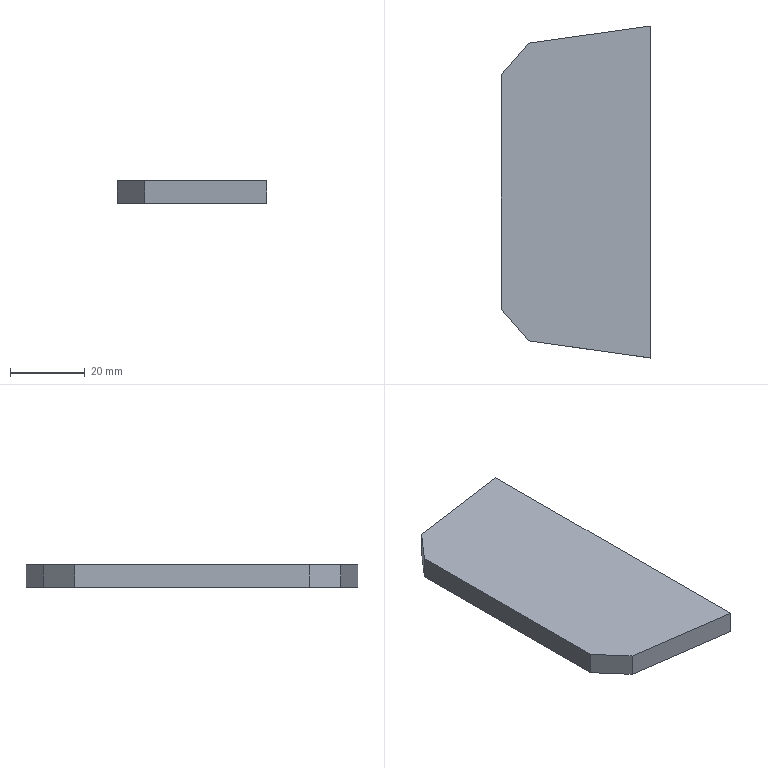Part | SolidWorks | features Extrusion 1 | 1 solid | 8 faces | box 40 x 88.903 x 6 mm | volume 19663 mm3 | plane 8
STEP:
#1=CARTESIAN_POINT('',(-4.,-5.549,0.));
#2=VERTEX_POINT('',#1);
#3=CARTESIAN_POINT('',(-4.,-94.451,0.));
#4=VERTEX_POINT('',#3);
#5=CARTESIAN_POINT('',(-4.,-5.549,0.));
#6=DIRECTION('',(0.,-1.,0.));
#7=VECTOR('',#6,1000.);
#8=LINE('',#5,#7);
#9=EDGE_CURVE('',#2,#4,#8,.T.);
#10=ORIENTED_EDGE('',*,*,#9,.F.);
#11=CARTESIAN_POINT('',(-4.,-5.549,6.));
#12=VERTEX_POINT('',#11);
#13=CARTESIAN_POINT('',(-4.,-5.549,6.));
#14=DIRECTION('',(0.,0.,-1.));
#15=VECTOR('',#14,1000.);
#16=LINE('',#13,#15);
#17=EDGE_CURVE('',#12,#2,#16,.T.);
#18=ORIENTED_EDGE('',*,*,#17,.F.);
#19=CARTESIAN_POINT('',(-4.,-94.451,6.));
#20=VERTEX_POINT('',#19);
#21=CARTESIAN_POINT('',(-4.,-5.549,6.));
#22=DIRECTION('',(0.,-1.,0.));
#23=VECTOR('',#22,1000.);
#24=LINE('',#21,#23);
#25=EDGE_CURVE('',#12,#20,#24,.T.);
#26=ORIENTED_EDGE('',*,*,#25,.T.);
#27=CARTESIAN_POINT('',(-4.,-94.451,6.));
#28=DIRECTION('',(0.,0.,-1.));
#29=VECTOR('',#28,1000.);
#30=LINE('',#27,#29);
#31=EDGE_CURVE('',#20,#4,#30,.T.);
#32=ORIENTED_EDGE('',*,*,#31,.T.);
#33=EDGE_LOOP('',(#10,#18,#26,#32));
#34=FACE_OUTER_BOUND('',#33,.T.);
#35=CARTESIAN_POINT('',(-4.,-5.549,6.));
#36=DIRECTION('',(1.,0.,0.));
#37=DIRECTION('',(0.,1.,0.));
#38=AXIS2_PLACEMENT_3D('',#35,#36,#37);
#39=PLANE('',#38);
#40=ADVANCED_FACE('',(#34),#39,.T.);
#41=CARTESIAN_POINT('',(-36.683,-10.142,0.));
#42=VERTEX_POINT('',#41);
#43=CARTESIAN_POINT('',(-36.683,-10.142,0.));
#44=DIRECTION('',(0.9903,0.1392,0.));
#45=VECTOR('',#44,1000.);
#46=LINE('',#43,#45);
#47=EDGE_CURVE('',#42,#2,#46,.T.);
#48=ORIENTED_EDGE('',*,*,#47,.F.);
#49=CARTESIAN_POINT('',(-36.683,-10.142,6.));
#50=VERTEX_POINT('',#49);
#51=CARTESIAN_POINT('',(-36.683,-10.142,6.));
#52=DIRECTION('',(0.,0.,-1.));
#53=VECTOR('',#52,1000.);
#54=LINE('',#51,#53);
#55=EDGE_CURVE('',#50,#42,#54,.T.);
#56=ORIENTED_EDGE('',*,*,#55,.F.);
#57=CARTESIAN_POINT('',(-36.683,-10.142,6.));
#58=DIRECTION('',(0.9903,0.1392,0.));
#59=VECTOR('',#58,1000.);
#60=LINE('',#57,#59);
#61=EDGE_CURVE('',#50,#12,#60,.T.);
#62=ORIENTED_EDGE('',*,*,#61,.T.);
#63=ORIENTED_EDGE('',*,*,#17,.T.);
#64=EDGE_LOOP('',(#48,#56,#62,#63));
#65=FACE_OUTER_BOUND('',#64,.T.);
#66=CARTESIAN_POINT('',(-36.683,-10.142,6.));
#67=DIRECTION('',(-0.1392,0.9903,0.));
#68=DIRECTION('',(-0.9903,-0.1392,0.));
#69=AXIS2_PLACEMENT_3D('',#66,#67,#68);
#70=PLANE('',#69);
#71=ADVANCED_FACE('',(#65),#70,.T.);
#72=CARTESIAN_POINT('',(-44.,-18.559,0.));
#73=VERTEX_POINT('',#72);
#74=CARTESIAN_POINT('',(-36.683,-10.142,0.));
#75=DIRECTION('',(-0.6561,-0.7547,0.));
#76=VECTOR('',#75,1000.);
#77=LINE('',#74,#76);
#78=EDGE_CURVE('',#42,#73,#77,.T.);
#79=ORIENTED_EDGE('',*,*,#78,.T.);
#80=CARTESIAN_POINT('',(-44.,-18.559,6.));
#81=VERTEX_POINT('',#80);
#82=CARTESIAN_POINT('',(-44.,-18.559,6.));
#83=DIRECTION('',(0.,0.,-1.));
#84=VECTOR('',#83,1000.);
#85=LINE('',#82,#84);
#86=EDGE_CURVE('',#81,#73,#85,.T.);
#87=ORIENTED_EDGE('',*,*,#86,.F.);
#88=CARTESIAN_POINT('',(-36.683,-10.142,6.));
#89=DIRECTION('',(-0.6561,-0.7547,0.));
#90=VECTOR('',#89,1000.);
#91=LINE('',#88,#90);
#92=EDGE_CURVE('',#50,#81,#91,.T.);
#93=ORIENTED_EDGE('',*,*,#92,.F.);
#94=ORIENTED_EDGE('',*,*,#55,.T.);
#95=EDGE_LOOP('',(#79,#87,#93,#94));
#96=FACE_OUTER_BOUND('',#95,.T.);
#97=CARTESIAN_POINT('',(-36.683,-10.142,6.));
#98=DIRECTION('',(0.7547,-0.6561,0.));
#99=DIRECTION('',(0.6561,0.7547,0.));
#100=AXIS2_PLACEMENT_3D('',#97,#98,#99);
#101=PLANE('',#100);
#102=ADVANCED_FACE('',(#96),#101,.F.);
#103=CARTESIAN_POINT('',(-44.,-81.441,0.));
#104=VERTEX_POINT('',#103);
#105=CARTESIAN_POINT('',(-44.,-81.441,0.));
#106=DIRECTION('',(0.,1.,0.));
#107=VECTOR('',#106,1000.);
#108=LINE('',#105,#107);
#109=EDGE_CURVE('',#104,#73,#108,.T.);
#110=ORIENTED_EDGE('',*,*,#109,.F.);
#111=CARTESIAN_POINT('',(-44.,-81.441,6.));
#112=VERTEX_POINT('',#111);
#113=CARTESIAN_POINT('',(-44.,-81.441,6.));
#114=DIRECTION('',(0.,0.,-1.));
#115=VECTOR('',#114,1000.);
#116=LINE('',#113,#115);
#117=EDGE_CURVE('',#112,#104,#116,.T.);
#118=ORIENTED_EDGE('',*,*,#117,.F.);
#119=CARTESIAN_POINT('',(-44.,-81.441,6.));
#120=DIRECTION('',(0.,1.,0.));
#121=VECTOR('',#120,1000.);
#122=LINE('',#119,#121);
#123=EDGE_CURVE('',#112,#81,#122,.T.);
#124=ORIENTED_EDGE('',*,*,#123,.T.);
#125=ORIENTED_EDGE('',*,*,#86,.T.);
#126=EDGE_LOOP('',(#110,#118,#124,#125));
#127=FACE_OUTER_BOUND('',#126,.T.);
#128=CARTESIAN_POINT('',(-44.,-81.441,6.));
#129=DIRECTION('',(-1.,0.,0.));
#130=DIRECTION('',(0.,0.,1.));
#131=AXIS2_PLACEMENT_3D('',#128,#129,#130);
#132=PLANE('',#131);
#133=ADVANCED_FACE('',(#127),#132,.T.);
#134=CARTESIAN_POINT('',(-36.683,-89.858,0.));
#135=VERTEX_POINT('',#134);
#136=CARTESIAN_POINT('',(-44.,-81.441,0.));
#137=DIRECTION('',(0.6561,-0.7547,0.));
#138=VECTOR('',#137,1000.);
#139=LINE('',#136,#138);
#140=EDGE_CURVE('',#104,#135,#139,.T.);
#141=ORIENTED_EDGE('',*,*,#140,.T.);
#142=CARTESIAN_POINT('',(-36.683,-89.858,6.));
#143=VERTEX_POINT('',#142);
#144=CARTESIAN_POINT('',(-36.683,-89.858,6.));
#145=DIRECTION('',(0.,0.,-1.));
#146=VECTOR('',#145,1000.);
#147=LINE('',#144,#146);
#148=EDGE_CURVE('',#143,#135,#147,.T.);
#149=ORIENTED_EDGE('',*,*,#148,.F.);
#150=CARTESIAN_POINT('',(-44.,-81.441,6.));
#151=DIRECTION('',(0.6561,-0.7547,0.));
#152=VECTOR('',#151,1000.);
#153=LINE('',#150,#152);
#154=EDGE_CURVE('',#112,#143,#153,.T.);
#155=ORIENTED_EDGE('',*,*,#154,.F.);
#156=ORIENTED_EDGE('',*,*,#117,.T.);
#157=EDGE_LOOP('',(#141,#149,#155,#156));
#158=FACE_OUTER_BOUND('',#157,.T.);
#159=CARTESIAN_POINT('',(-44.,-81.441,6.));
#160=DIRECTION('',(0.7547,0.6561,0.));
#161=DIRECTION('',(-0.6561,0.7547,0.));
#162=AXIS2_PLACEMENT_3D('',#159,#160,#161);
#163=PLANE('',#162);
#164=ADVANCED_FACE('',(#158),#163,.F.);
#165=CARTESIAN_POINT('',(-4.,-94.451,0.));
#166=DIRECTION('',(-0.9903,0.1392,0.));
#167=VECTOR('',#166,1000.);
#168=LINE('',#165,#167);
#169=EDGE_CURVE('',#4,#135,#168,.T.);
#170=ORIENTED_EDGE('',*,*,#169,.F.);
#171=ORIENTED_EDGE('',*,*,#31,.F.);
#172=CARTESIAN_POINT('',(-4.,-94.451,6.));
#173=DIRECTION('',(-0.9903,0.1392,0.));
#174=VECTOR('',#173,1000.);
#175=LINE('',#172,#174);
#176=EDGE_CURVE('',#20,#143,#175,.T.);
#177=ORIENTED_EDGE('',*,*,#176,.T.);
#178=ORIENTED_EDGE('',*,*,#148,.T.);
#179=EDGE_LOOP('',(#170,#171,#177,#178));
#180=FACE_OUTER_BOUND('',#179,.T.);
#181=CARTESIAN_POINT('',(-4.,-94.451,6.));
#182=DIRECTION('',(-0.1392,-0.9903,0.));
#183=DIRECTION('',(0.9903,-0.1392,0.));
#184=AXIS2_PLACEMENT_3D('',#181,#182,#183);
#185=PLANE('',#184);
#186=ADVANCED_FACE('',(#180),#185,.T.);
#187=ORIENTED_EDGE('',*,*,#25,.F.);
#188=ORIENTED_EDGE('',*,*,#61,.F.);
#189=ORIENTED_EDGE('',*,*,#92,.T.);
#190=ORIENTED_EDGE('',*,*,#123,.F.);
#191=ORIENTED_EDGE('',*,*,#154,.T.);
#192=ORIENTED_EDGE('',*,*,#176,.F.);
#193=EDGE_LOOP('',(#187,#188,#189,#190,#191,#192));
#194=FACE_OUTER_BOUND('',#193,.T.);
#195=CARTESIAN_POINT('',(0.,0.,6.));
#196=DIRECTION('',(0.,0.,-1.));
#197=DIRECTION('',(-1.,0.,0.));
#198=AXIS2_PLACEMENT_3D('',#195,#196,#197);
#199=PLANE('',#198);
#200=ADVANCED_FACE('',(#194),#199,.F.);
#201=ORIENTED_EDGE('',*,*,#9,.T.);
#202=ORIENTED_EDGE('',*,*,#169,.T.);
#203=ORIENTED_EDGE('',*,*,#140,.F.);
#204=ORIENTED_EDGE('',*,*,#109,.T.);
#205=ORIENTED_EDGE('',*,*,#78,.F.);
#206=ORIENTED_EDGE('',*,*,#47,.T.);
#207=EDGE_LOOP('',(#201,#202,#203,#204,#205,#206));
#208=FACE_OUTER_BOUND('',#207,.T.);
#209=CARTESIAN_POINT('',(0.,0.,0.));
#210=DIRECTION('',(0.,0.,-1.));
#211=DIRECTION('',(-1.,0.,0.));
#212=AXIS2_PLACEMENT_3D('',#209,#210,#211);
#213=PLANE('',#212);
#214=ADVANCED_FACE('',(#208),#213,.T.);
#215=CLOSED_SHELL('',(#40,#71,#102,#133,#164,#186,#200,#214));
#216=MANIFOLD_SOLID_BREP('',#215);
#217=CARTESIAN_POINT('',(0.,0.,0.));
#218=DIRECTION('',(0.,0.,1.));
#219=DIRECTION('',(1.,0.,0.));
#220=AXIS2_PLACEMENT_3D('',#217,#218,#219);
#221=(LENGTH_UNIT()NAMED_UNIT(*)SI_UNIT(.MILLI.,.METRE.));
#222=UNCERTAINTY_MEASURE_WITH_UNIT(LENGTH_MEASURE(0.00001),#221,'','');
#223=(NAMED_UNIT(*)PLANE_ANGLE_UNIT()SI_UNIT($,.RADIAN.));
#224=(NAMED_UNIT(*)SI_UNIT($,.STERADIAN.)SOLID_ANGLE_UNIT());
#225=(GEOMETRIC_REPRESENTATION_CONTEXT(3)GLOBAL_UNCERTAINTY_ASSIGNED_CONTEXT((#222))GLOBAL_UNIT_ASSIGNED_CONTEXT((#221,#223,#224))REPRESENTATION_CONTEXT('',''));
#226=ADVANCED_BREP_SHAPE_REPRESENTATION('',(#216,#220),#225);